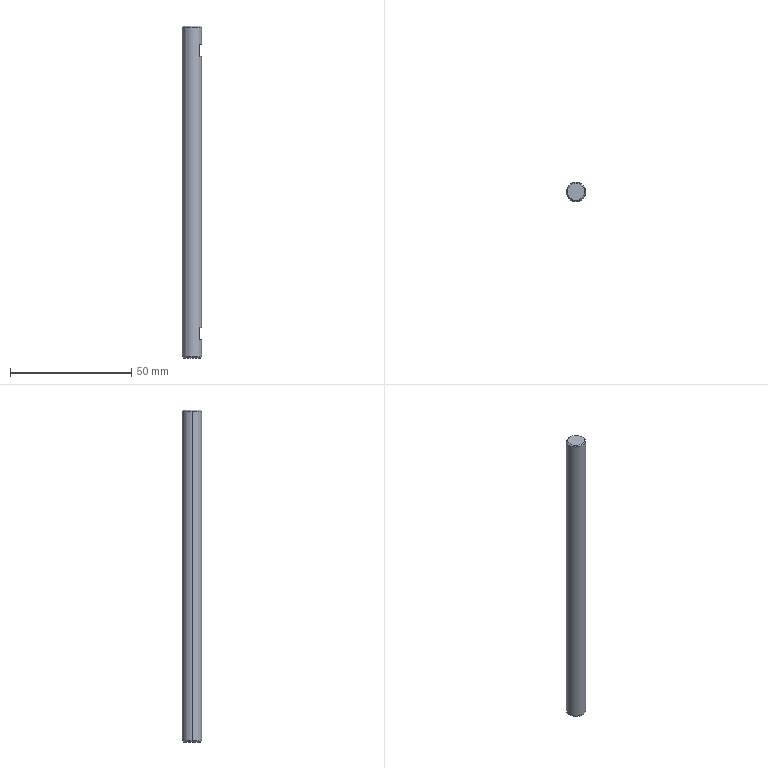Part | STEP file | 11-FG-B00411 | 1 solid | 14 faces | box 8 x 8 x 137 mm | volume 6844 mm3 | plane 8 | cone 4 | cylinder 2 | commonest cylinder face diameters 8 x2
STEP:
#1=CARTESIAN_POINT('',(3.5,0.,137.));
#2=VERTEX_POINT('',#1);
#3=CARTESIAN_POINT('',(-3.5,0.,137.));
#4=VERTEX_POINT('',#3);
#5=CARTESIAN_POINT('',(0.,0.,137.));
#6=DIRECTION('',(0.,0.,1.));
#7=DIRECTION('',(1.,0.,0.));
#8=AXIS2_PLACEMENT_3D('',#5,#6,#7);
#9=CIRCLE('',#8,3.5);
#10=EDGE_CURVE('',#2,#4,#9,.T.);
#11=ORIENTED_EDGE('',*,*,#10,.F.);
#12=CARTESIAN_POINT('',(4.,0.,136.5));
#13=VERTEX_POINT('',#12);
#14=CARTESIAN_POINT('',(3.5,0.,137.));
#15=DIRECTION('',(0.7071,0.,-0.7071));
#16=VECTOR('',#15,1000.);
#17=LINE('',#14,#16);
#18=EDGE_CURVE('',#2,#13,#17,.T.);
#19=ORIENTED_EDGE('',*,*,#18,.T.);
#20=CARTESIAN_POINT('',(-4.,0.,136.5));
#21=VERTEX_POINT('',#20);
#22=CARTESIAN_POINT('',(0.,0.,136.5));
#23=DIRECTION('',(0.,0.,-1.));
#24=DIRECTION('',(1.,0.,0.));
#25=AXIS2_PLACEMENT_3D('',#22,#23,#24);
#26=CIRCLE('',#25,4.);
#27=EDGE_CURVE('',#21,#13,#26,.T.);
#28=ORIENTED_EDGE('',*,*,#27,.F.);
#29=CARTESIAN_POINT('',(-3.5,0.,137.));
#30=DIRECTION('',(-0.7071,0.,-0.7071));
#31=VECTOR('',#30,1000.);
#32=LINE('',#29,#31);
#33=EDGE_CURVE('',#4,#21,#32,.T.);
#34=ORIENTED_EDGE('',*,*,#33,.F.);
#35=EDGE_LOOP('',(#11,#19,#28,#34));
#36=FACE_OUTER_BOUND('',#35,.T.);
#37=CARTESIAN_POINT('',(0.,0.,137.));
#38=DIRECTION('',(0.,0.,-1.));
#39=DIRECTION('',(-1.,0.,0.));
#40=AXIS2_PLACEMENT_3D('',#37,#38,#39);
#41=CONICAL_SURFACE('',#40,3.5,0.7854);
#42=ADVANCED_FACE('',(#36),#41,.T.);
#43=CARTESIAN_POINT('',(-3.5,0.,0.));
#44=VERTEX_POINT('',#43);
#45=CARTESIAN_POINT('',(3.5,0.,0.));
#46=VERTEX_POINT('',#45);
#47=CARTESIAN_POINT('',(0.,0.,0.));
#48=DIRECTION('',(0.,0.,-1.));
#49=DIRECTION('',(1.,0.,0.));
#50=AXIS2_PLACEMENT_3D('',#47,#48,#49);
#51=CIRCLE('',#50,3.5);
#52=EDGE_CURVE('',#44,#46,#51,.T.);
#53=ORIENTED_EDGE('',*,*,#52,.F.);
#54=CARTESIAN_POINT('',(-4.,0.,0.5));
#55=VERTEX_POINT('',#54);
#56=CARTESIAN_POINT('',(-4.,0.,0.5));
#57=DIRECTION('',(-0.7071,0.,0.7071));
#58=VECTOR('',#57,1000.);
#59=LINE('',#56,#58);
#60=EDGE_CURVE('',#44,#55,#59,.T.);
#61=ORIENTED_EDGE('',*,*,#60,.T.);
#62=CARTESIAN_POINT('',(4.,0.,0.5));
#63=VERTEX_POINT('',#62);
#64=CARTESIAN_POINT('',(0.,0.,0.5));
#65=DIRECTION('',(0.,0.,1.));
#66=DIRECTION('',(1.,0.,0.));
#67=AXIS2_PLACEMENT_3D('',#64,#65,#66);
#68=CIRCLE('',#67,4.);
#69=EDGE_CURVE('',#63,#55,#68,.T.);
#70=ORIENTED_EDGE('',*,*,#69,.F.);
#71=CARTESIAN_POINT('',(4.,0.,0.5));
#72=DIRECTION('',(0.7071,0.,0.7071));
#73=VECTOR('',#72,1000.);
#74=LINE('',#71,#73);
#75=EDGE_CURVE('',#46,#63,#74,.T.);
#76=ORIENTED_EDGE('',*,*,#75,.F.);
#77=EDGE_LOOP('',(#53,#61,#70,#76));
#78=FACE_OUTER_BOUND('',#77,.T.);
#79=CARTESIAN_POINT('',(0.,0.,0.5));
#80=DIRECTION('',(0.,0.,1.));
#81=DIRECTION('',(1.,0.,0.));
#82=AXIS2_PLACEMENT_3D('',#79,#80,#81);
#83=CONICAL_SURFACE('',#82,4.,0.7854);
#84=ADVANCED_FACE('',(#78),#83,.T.);
#85=ORIENTED_EDGE('',*,*,#27,.T.);
#86=CARTESIAN_POINT('',(4.,0.,129.5));
#87=VERTEX_POINT('',#86);
#88=CARTESIAN_POINT('',(4.,0.,137.));
#89=DIRECTION('',(0.,0.,-1.));
#90=VECTOR('',#89,1000.);
#91=LINE('',#88,#90);
#92=EDGE_CURVE('',#13,#87,#91,.T.);
#93=ORIENTED_EDGE('',*,*,#92,.T.);
#94=CARTESIAN_POINT('',(3.,2.646,129.5));
#95=VERTEX_POINT('',#94);
#96=CARTESIAN_POINT('',(0.,0.,129.5));
#97=DIRECTION('',(0.,0.,-1.));
#98=DIRECTION('',(-1.,0.,0.));
#99=AXIS2_PLACEMENT_3D('',#96,#97,#98);
#100=CIRCLE('',#99,4.);
#101=EDGE_CURVE('',#95,#87,#100,.T.);
#102=ORIENTED_EDGE('',*,*,#101,.F.);
#103=CARTESIAN_POINT('',(3.,2.646,124.5));
#104=VERTEX_POINT('',#103);
#105=CARTESIAN_POINT('',(3.,2.646,137.));
#106=DIRECTION('',(0.,0.,1.));
#107=VECTOR('',#106,1000.);
#108=LINE('',#105,#107);
#109=EDGE_CURVE('',#104,#95,#108,.T.);
#110=ORIENTED_EDGE('',*,*,#109,.F.);
#111=CARTESIAN_POINT('',(4.,0.,124.5));
#112=VERTEX_POINT('',#111);
#113=CARTESIAN_POINT('',(0.,0.,124.5));
#114=DIRECTION('',(0.,0.,1.));
#115=DIRECTION('',(1.,0.,0.));
#116=AXIS2_PLACEMENT_3D('',#113,#114,#115);
#117=CIRCLE('',#116,4.);
#118=EDGE_CURVE('',#112,#104,#117,.T.);
#119=ORIENTED_EDGE('',*,*,#118,.F.);
#120=CARTESIAN_POINT('',(4.,0.,12.5));
#121=VERTEX_POINT('',#120);
#122=CARTESIAN_POINT('',(4.,0.,137.));
#123=DIRECTION('',(0.,0.,-1.));
#124=VECTOR('',#123,1000.);
#125=LINE('',#122,#124);
#126=EDGE_CURVE('',#112,#121,#125,.T.);
#127=ORIENTED_EDGE('',*,*,#126,.T.);
#128=CARTESIAN_POINT('',(3.,2.646,12.5));
#129=VERTEX_POINT('',#128);
#130=CARTESIAN_POINT('',(0.,0.,12.5));
#131=DIRECTION('',(0.,0.,-1.));
#132=DIRECTION('',(-1.,0.,0.));
#133=AXIS2_PLACEMENT_3D('',#130,#131,#132);
#134=CIRCLE('',#133,4.);
#135=EDGE_CURVE('',#129,#121,#134,.T.);
#136=ORIENTED_EDGE('',*,*,#135,.F.);
#137=CARTESIAN_POINT('',(3.,2.646,7.5));
#138=VERTEX_POINT('',#137);
#139=CARTESIAN_POINT('',(3.,2.646,137.));
#140=DIRECTION('',(0.,0.,1.));
#141=VECTOR('',#140,1000.);
#142=LINE('',#139,#141);
#143=EDGE_CURVE('',#138,#129,#142,.T.);
#144=ORIENTED_EDGE('',*,*,#143,.F.);
#145=CARTESIAN_POINT('',(4.,0.,7.5));
#146=VERTEX_POINT('',#145);
#147=CARTESIAN_POINT('',(0.,0.,7.5));
#148=DIRECTION('',(0.,0.,1.));
#149=DIRECTION('',(0.,-1.,0.));
#150=AXIS2_PLACEMENT_3D('',#147,#148,#149);
#151=CIRCLE('',#150,4.);
#152=EDGE_CURVE('',#146,#138,#151,.T.);
#153=ORIENTED_EDGE('',*,*,#152,.F.);
#154=CARTESIAN_POINT('',(4.,0.,137.));
#155=DIRECTION('',(0.,0.,-1.));
#156=VECTOR('',#155,1000.);
#157=LINE('',#154,#156);
#158=EDGE_CURVE('',#146,#63,#157,.T.);
#159=ORIENTED_EDGE('',*,*,#158,.T.);
#160=ORIENTED_EDGE('',*,*,#69,.T.);
#161=CARTESIAN_POINT('',(-4.,0.,137.));
#162=DIRECTION('',(0.,0.,-1.));
#163=VECTOR('',#162,1000.);
#164=LINE('',#161,#163);
#165=EDGE_CURVE('',#21,#55,#164,.T.);
#166=ORIENTED_EDGE('',*,*,#165,.F.);
#167=EDGE_LOOP('',(#85,#93,#102,#110,#119,#127,#136,#144,#153,#159,#160,#166));
#168=FACE_OUTER_BOUND('',#167,.T.);
#169=CARTESIAN_POINT('',(0.,0.,137.));
#170=DIRECTION('',(0.,0.,-1.));
#171=DIRECTION('',(-1.,0.,0.));
#172=AXIS2_PLACEMENT_3D('',#169,#170,#171);
#173=CYLINDRICAL_SURFACE('',#172,4.);
#174=ADVANCED_FACE('',(#168),#173,.T.);
#175=ORIENTED_EDGE('',*,*,#92,.F.);
#176=CARTESIAN_POINT('',(0.,0.,136.5));
#177=DIRECTION('',(0.,0.,-1.));
#178=DIRECTION('',(1.,0.,0.));
#179=AXIS2_PLACEMENT_3D('',#176,#177,#178);
#180=CIRCLE('',#179,4.);
#181=EDGE_CURVE('',#13,#21,#180,.T.);
#182=ORIENTED_EDGE('',*,*,#181,.T.);
#183=ORIENTED_EDGE('',*,*,#165,.T.);
#184=CARTESIAN_POINT('',(0.,0.,0.5));
#185=DIRECTION('',(0.,0.,1.));
#186=DIRECTION('',(1.,0.,0.));
#187=AXIS2_PLACEMENT_3D('',#184,#185,#186);
#188=CIRCLE('',#187,4.);
#189=EDGE_CURVE('',#55,#63,#188,.T.);
#190=ORIENTED_EDGE('',*,*,#189,.T.);
#191=ORIENTED_EDGE('',*,*,#158,.F.);
#192=CARTESIAN_POINT('',(3.,-2.646,7.5));
#193=VERTEX_POINT('',#192);
#194=CARTESIAN_POINT('',(0.,0.,7.5));
#195=DIRECTION('',(0.,0.,1.));
#196=DIRECTION('',(0.,-1.,0.));
#197=AXIS2_PLACEMENT_3D('',#194,#195,#196);
#198=CIRCLE('',#197,4.);
#199=EDGE_CURVE('',#193,#146,#198,.T.);
#200=ORIENTED_EDGE('',*,*,#199,.F.);
#201=CARTESIAN_POINT('',(3.,-2.646,12.5));
#202=VERTEX_POINT('',#201);
#203=CARTESIAN_POINT('',(3.,-2.646,137.));
#204=DIRECTION('',(0.,0.,-1.));
#205=VECTOR('',#204,1000.);
#206=LINE('',#203,#205);
#207=EDGE_CURVE('',#202,#193,#206,.T.);
#208=ORIENTED_EDGE('',*,*,#207,.F.);
#209=CARTESIAN_POINT('',(0.,0.,12.5));
#210=DIRECTION('',(0.,0.,-1.));
#211=DIRECTION('',(-1.,0.,0.));
#212=AXIS2_PLACEMENT_3D('',#209,#210,#211);
#213=CIRCLE('',#212,4.);
#214=EDGE_CURVE('',#121,#202,#213,.T.);
#215=ORIENTED_EDGE('',*,*,#214,.F.);
#216=ORIENTED_EDGE('',*,*,#126,.F.);
#217=CARTESIAN_POINT('',(3.,-2.646,124.5));
#218=VERTEX_POINT('',#217);
#219=CARTESIAN_POINT('',(0.,0.,124.5));
#220=DIRECTION('',(0.,0.,1.));
#221=DIRECTION('',(1.,0.,0.));
#222=AXIS2_PLACEMENT_3D('',#219,#220,#221);
#223=CIRCLE('',#222,4.);
#224=EDGE_CURVE('',#218,#112,#223,.T.);
#225=ORIENTED_EDGE('',*,*,#224,.F.);
#226=CARTESIAN_POINT('',(3.,-2.646,129.5));
#227=VERTEX_POINT('',#226);
#228=CARTESIAN_POINT('',(3.,-2.646,137.));
#229=DIRECTION('',(0.,0.,-1.));
#230=VECTOR('',#229,1000.);
#231=LINE('',#228,#230);
#232=EDGE_CURVE('',#227,#218,#231,.T.);
#233=ORIENTED_EDGE('',*,*,#232,.F.);
#234=CARTESIAN_POINT('',(0.,0.,129.5));
#235=DIRECTION('',(0.,0.,-1.));
#236=DIRECTION('',(-1.,0.,0.));
#237=AXIS2_PLACEMENT_3D('',#234,#235,#236);
#238=CIRCLE('',#237,4.);
#239=EDGE_CURVE('',#87,#227,#238,.T.);
#240=ORIENTED_EDGE('',*,*,#239,.F.);
#241=EDGE_LOOP('',(#175,#182,#183,#190,#191,#200,#208,#215,#216,#225,#233,#240));
#242=FACE_OUTER_BOUND('',#241,.T.);
#243=CARTESIAN_POINT('',(0.,0.,137.));
#244=DIRECTION('',(0.,0.,-1.));
#245=DIRECTION('',(-1.,0.,0.));
#246=AXIS2_PLACEMENT_3D('',#243,#244,#245);
#247=CYLINDRICAL_SURFACE('',#246,4.);
#248=ADVANCED_FACE('',(#242),#247,.T.);
#249=CARTESIAN_POINT('',(0.,0.,137.));
#250=DIRECTION('',(0.,0.,1.));
#251=DIRECTION('',(1.,0.,0.));
#252=AXIS2_PLACEMENT_3D('',#249,#250,#251);
#253=CIRCLE('',#252,3.5);
#254=EDGE_CURVE('',#4,#2,#253,.T.);
#255=ORIENTED_EDGE('',*,*,#254,.T.);
#256=ORIENTED_EDGE('',*,*,#10,.T.);
#257=EDGE_LOOP('',(#255,#256));
#258=FACE_OUTER_BOUND('',#257,.T.);
#259=CARTESIAN_POINT('',(0.,0.,137.));
#260=DIRECTION('',(0.,0.,1.));
#261=DIRECTION('',(1.,0.,0.));
#262=AXIS2_PLACEMENT_3D('',#259,#260,#261);
#263=PLANE('',#262);
#264=ADVANCED_FACE('',(#258),#263,.T.);
#265=CARTESIAN_POINT('',(0.,0.,0.));
#266=DIRECTION('',(0.,0.,-1.));
#267=DIRECTION('',(1.,0.,0.));
#268=AXIS2_PLACEMENT_3D('',#265,#266,#267);
#269=CIRCLE('',#268,3.5);
#270=EDGE_CURVE('',#46,#44,#269,.T.);
#271=ORIENTED_EDGE('',*,*,#270,.T.);
#272=ORIENTED_EDGE('',*,*,#52,.T.);
#273=EDGE_LOOP('',(#271,#272));
#274=FACE_OUTER_BOUND('',#273,.T.);
#275=CARTESIAN_POINT('',(0.,0.,0.));
#276=DIRECTION('',(0.,0.,1.));
#277=DIRECTION('',(1.,0.,0.));
#278=AXIS2_PLACEMENT_3D('',#275,#276,#277);
#279=PLANE('',#278);
#280=ADVANCED_FACE('',(#274),#279,.F.);
#281=ORIENTED_EDGE('',*,*,#101,.T.);
#282=ORIENTED_EDGE('',*,*,#239,.T.);
#283=CARTESIAN_POINT('',(3.,5.701,129.5));
#284=DIRECTION('',(0.,-1.,0.));
#285=VECTOR('',#284,1000.);
#286=LINE('',#283,#285);
#287=EDGE_CURVE('',#95,#227,#286,.T.);
#288=ORIENTED_EDGE('',*,*,#287,.F.);
#289=EDGE_LOOP('',(#281,#282,#288));
#290=FACE_OUTER_BOUND('',#289,.T.);
#291=CARTESIAN_POINT('',(108.,5.701,129.5));
#292=DIRECTION('',(0.,0.,-1.));
#293=DIRECTION('',(-1.,0.,0.));
#294=AXIS2_PLACEMENT_3D('',#291,#292,#293);
#295=PLANE('',#294);
#296=ADVANCED_FACE('',(#290),#295,.T.);
#297=ORIENTED_EDGE('',*,*,#224,.T.);
#298=ORIENTED_EDGE('',*,*,#118,.T.);
#299=CARTESIAN_POINT('',(3.,5.701,124.5));
#300=DIRECTION('',(0.,1.,0.));
#301=VECTOR('',#300,1000.);
#302=LINE('',#299,#301);
#303=EDGE_CURVE('',#218,#104,#302,.T.);
#304=ORIENTED_EDGE('',*,*,#303,.F.);
#305=EDGE_LOOP('',(#297,#298,#304));
#306=FACE_OUTER_BOUND('',#305,.T.);
#307=CARTESIAN_POINT('',(108.,5.701,124.5));
#308=DIRECTION('',(0.,0.,1.));
#309=DIRECTION('',(1.,0.,0.));
#310=AXIS2_PLACEMENT_3D('',#307,#308,#309);
#311=PLANE('',#310);
#312=ADVANCED_FACE('',(#306),#311,.T.);
#313=ORIENTED_EDGE('',*,*,#232,.T.);
#314=ORIENTED_EDGE('',*,*,#303,.T.);
#315=ORIENTED_EDGE('',*,*,#109,.T.);
#316=ORIENTED_EDGE('',*,*,#287,.T.);
#317=EDGE_LOOP('',(#313,#314,#315,#316));
#318=FACE_OUTER_BOUND('',#317,.T.);
#319=CARTESIAN_POINT('',(3.,-5.543,129.5));
#320=DIRECTION('',(1.,0.,0.));
#321=DIRECTION('',(0.,0.,-1.));
#322=AXIS2_PLACEMENT_3D('',#319,#320,#321);
#323=PLANE('',#322);
#324=ADVANCED_FACE('',(#318),#323,.T.);
#325=ORIENTED_EDGE('',*,*,#135,.T.);
#326=ORIENTED_EDGE('',*,*,#214,.T.);
#327=CARTESIAN_POINT('',(3.,9.219,12.5));
#328=DIRECTION('',(0.,-1.,0.));
#329=VECTOR('',#328,1000.);
#330=LINE('',#327,#329);
#331=EDGE_CURVE('',#129,#202,#330,.T.);
#332=ORIENTED_EDGE('',*,*,#331,.F.);
#333=EDGE_LOOP('',(#325,#326,#332));
#334=FACE_OUTER_BOUND('',#333,.T.);
#335=CARTESIAN_POINT('',(108.,9.219,12.5));
#336=DIRECTION('',(0.,0.,-1.));
#337=DIRECTION('',(-1.,0.,0.));
#338=AXIS2_PLACEMENT_3D('',#335,#336,#337);
#339=PLANE('',#338);
#340=ADVANCED_FACE('',(#334),#339,.T.);
#341=ORIENTED_EDGE('',*,*,#199,.T.);
#342=ORIENTED_EDGE('',*,*,#152,.T.);
#343=CARTESIAN_POINT('',(3.,9.219,7.5));
#344=DIRECTION('',(0.,1.,0.));
#345=VECTOR('',#344,1000.);
#346=LINE('',#343,#345);
#347=EDGE_CURVE('',#193,#138,#346,.T.);
#348=ORIENTED_EDGE('',*,*,#347,.F.);
#349=EDGE_LOOP('',(#341,#342,#348));
#350=FACE_OUTER_BOUND('',#349,.T.);
#351=CARTESIAN_POINT('',(108.,9.219,7.5));
#352=DIRECTION('',(0.,0.,1.));
#353=DIRECTION('',(0.,-1.,0.));
#354=AXIS2_PLACEMENT_3D('',#351,#352,#353);
#355=PLANE('',#354);
#356=ADVANCED_FACE('',(#350),#355,.T.);
#357=ORIENTED_EDGE('',*,*,#207,.T.);
#358=ORIENTED_EDGE('',*,*,#347,.T.);
#359=ORIENTED_EDGE('',*,*,#143,.T.);
#360=ORIENTED_EDGE('',*,*,#331,.T.);
#361=EDGE_LOOP('',(#357,#358,#359,#360));
#362=FACE_OUTER_BOUND('',#361,.T.);
#363=CARTESIAN_POINT('',(3.,-7.736,12.5));
#364=DIRECTION('',(1.,0.,0.));
#365=DIRECTION('',(0.,0.,-1.));
#366=AXIS2_PLACEMENT_3D('',#363,#364,#365);
#367=PLANE('',#366);
#368=ADVANCED_FACE('',(#362),#367,.T.);
#369=ORIENTED_EDGE('',*,*,#60,.F.);
#370=ORIENTED_EDGE('',*,*,#270,.F.);
#371=ORIENTED_EDGE('',*,*,#75,.T.);
#372=ORIENTED_EDGE('',*,*,#189,.F.);
#373=EDGE_LOOP('',(#369,#370,#371,#372));
#374=FACE_OUTER_BOUND('',#373,.T.);
#375=CARTESIAN_POINT('',(0.,0.,0.5));
#376=DIRECTION('',(0.,0.,1.));
#377=DIRECTION('',(1.,0.,0.));
#378=AXIS2_PLACEMENT_3D('',#375,#376,#377);
#379=CONICAL_SURFACE('',#378,4.,0.7854);
#380=ADVANCED_FACE('',(#374),#379,.T.);
#381=ORIENTED_EDGE('',*,*,#18,.F.);
#382=ORIENTED_EDGE('',*,*,#254,.F.);
#383=ORIENTED_EDGE('',*,*,#33,.T.);
#384=ORIENTED_EDGE('',*,*,#181,.F.);
#385=EDGE_LOOP('',(#381,#382,#383,#384));
#386=FACE_OUTER_BOUND('',#385,.T.);
#387=CARTESIAN_POINT('',(0.,0.,137.));
#388=DIRECTION('',(0.,0.,-1.));
#389=DIRECTION('',(-1.,0.,0.));
#390=AXIS2_PLACEMENT_3D('',#387,#388,#389);
#391=CONICAL_SURFACE('',#390,3.5,0.7854);
#392=ADVANCED_FACE('',(#386),#391,.T.);
#393=CLOSED_SHELL('',(#42,#84,#174,#248,#264,#280,#296,#312,#324,#340,#356,#368,#380,#392));
#394=MANIFOLD_SOLID_BREP('',#393);
#395=CARTESIAN_POINT('',(0.,0.,0.));
#396=DIRECTION('',(0.,0.,1.));
#397=DIRECTION('',(1.,0.,0.));
#398=AXIS2_PLACEMENT_3D('',#395,#396,#397);
#399=(LENGTH_UNIT()NAMED_UNIT(*)SI_UNIT(.MILLI.,.METRE.));
#400=UNCERTAINTY_MEASURE_WITH_UNIT(LENGTH_MEASURE(0.00001),#399,'','');
#401=(NAMED_UNIT(*)PLANE_ANGLE_UNIT()SI_UNIT($,.RADIAN.));
#402=(NAMED_UNIT(*)SI_UNIT($,.STERADIAN.)SOLID_ANGLE_UNIT());
#403=(GEOMETRIC_REPRESENTATION_CONTEXT(3)GLOBAL_UNCERTAINTY_ASSIGNED_CONTEXT((#400))GLOBAL_UNIT_ASSIGNED_CONTEXT((#399,#401,#402))REPRESENTATION_CONTEXT('',''));
#404=ADVANCED_BREP_SHAPE_REPRESENTATION('',(#394,#398),#403);